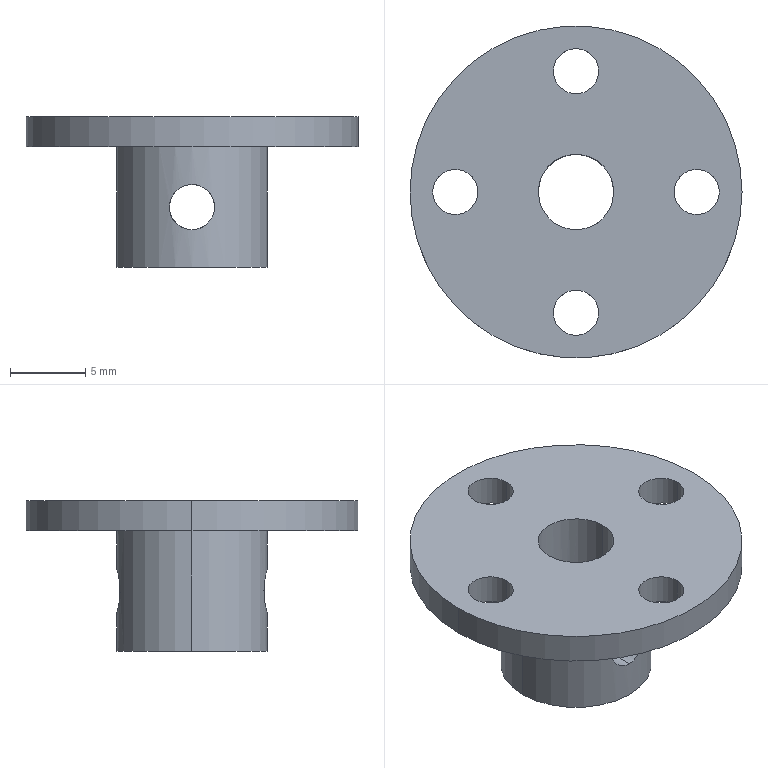Part | SolidWorks | features ICE 4, Extrusion 1 | 1 solid | 21 faces | box 22 x 22 x 10 mm | volume 1099 mm3 | cylinder 18 | plane 3 | commonest cylinder face diameters 3 x12 5 x2 10 x2 22 x2
STEP:
#1=CARTESIAN_POINT('',(0.,-5.,-5.5));
#2=VERTEX_POINT('',#1);
#3=CARTESIAN_POINT('',(0.,-5.,-2.5));
#4=VERTEX_POINT('',#3);
#5=CARTESIAN_POINT('',(0.,-5.,-5.5));
#6=CARTESIAN_POINT('',(-0.1965,-5.,-5.5));
#7=CARTESIAN_POINT('',(-0.3949,-4.988,-5.46));
#8=CARTESIAN_POINT('',(-0.6661,-4.956,-5.348));
#9=CARTESIAN_POINT('',(-0.7539,-4.944,-5.3));
#10=CARTESIAN_POINT('',(-0.9162,-4.916,-5.192));
#11=CARTESIAN_POINT('',(-0.9913,-4.901,-5.13));
#12=CARTESIAN_POINT('',(-1.199,-4.856,-4.922));
#13=CARTESIAN_POINT('',(-1.309,-4.826,-4.759));
#14=CARTESIAN_POINT('',(-1.423,-4.793,-4.485));
#15=CARTESIAN_POINT('',(-1.451,-4.785,-4.391));
#16=CARTESIAN_POINT('',(-1.49,-4.773,-4.199));
#17=CARTESIAN_POINT('',(-1.5,-4.77,-4.099));
#18=CARTESIAN_POINT('',(-1.5,-4.77,-3.901));
#19=CARTESIAN_POINT('',(-1.49,-4.773,-3.804));
#20=CARTESIAN_POINT('',(-1.452,-4.785,-3.61));
#21=CARTESIAN_POINT('',(-1.423,-4.793,-3.515));
#22=CARTESIAN_POINT('',(-1.31,-4.826,-3.244));
#23=CARTESIAN_POINT('',(-1.199,-4.856,-3.077));
#24=CARTESIAN_POINT('',(-0.9924,-4.901,-2.871));
#25=CARTESIAN_POINT('',(-0.9159,-4.916,-2.808));
#26=CARTESIAN_POINT('',(-0.7533,-4.944,-2.699));
#27=CARTESIAN_POINT('',(-0.6674,-4.956,-2.653));
#28=CARTESIAN_POINT('',(-0.4865,-4.977,-2.578));
#29=CARTESIAN_POINT('',(-0.3907,-4.986,-2.548));
#30=CARTESIAN_POINT('',(-0.1978,-4.997,-2.51));
#31=CARTESIAN_POINT('',(-0.0997,-5.,-2.5));
#32=CARTESIAN_POINT('',(0.,-5.,-2.5));
#33=B_SPLINE_CURVE_WITH_KNOTS('',3,(#5,#6,#7,#8,#9,#10,#11,#12,#13,#14,#15,#16,#17,#18,#19,#20,#21,#22,#23,#24,#25,#26,#27,#28,#29,#30,#31,#32),.UNSPECIFIED.,.F.,.F.,(4,2,2,2,2,2,2,2,2,2,2,2,2,4),(0.004717,0.005306,0.005601,0.005896,0.006485,0.00678,0.007075,0.00737,0.007664,0.008254,0.008549,0.008843,0.009138,0.009433),.UNSPECIFIED.);
#34=EDGE_CURVE('',#2,#4,#33,.T.);
#35=ORIENTED_EDGE('',*,*,#34,.F.);
#36=CARTESIAN_POINT('',(0.,-2.5,-5.5));
#37=VERTEX_POINT('',#36);
#38=CARTESIAN_POINT('',(0.,-7.,-5.5));
#39=DIRECTION('',(0.,1.,0.));
#40=VECTOR('',#39,1000.);
#41=LINE('',#38,#40);
#42=EDGE_CURVE('',#2,#37,#41,.T.);
#43=ORIENTED_EDGE('',*,*,#42,.T.);
#44=CARTESIAN_POINT('',(0.,-2.5,-2.5));
#45=VERTEX_POINT('',#44);
#46=CARTESIAN_POINT('',(0.,-2.5,-2.5));
#47=CARTESIAN_POINT('',(-0.1019,-2.5,-2.5));
#48=CARTESIAN_POINT('',(-0.2016,-2.494,-2.51));
#49=CARTESIAN_POINT('',(-0.397,-2.47,-2.55));
#50=CARTESIAN_POINT('',(-0.4936,-2.453,-2.58));
#51=CARTESIAN_POINT('',(-0.7651,-2.387,-2.695));
#52=CARTESIAN_POINT('',(-0.9278,-2.326,-2.806));
#53=CARTESIAN_POINT('',(-1.197,-2.2,-3.076));
#54=CARTESIAN_POINT('',(-1.306,-2.133,-3.238));
#55=CARTESIAN_POINT('',(-1.458,-2.033,-3.596));
#56=CARTESIAN_POINT('',(-1.5,-2.,-3.796));
#57=CARTESIAN_POINT('',(-1.5,-2.,-4.101));
#58=CARTESIAN_POINT('',(-1.49,-2.008,-4.201));
#59=CARTESIAN_POINT('',(-1.45,-2.037,-4.397));
#60=CARTESIAN_POINT('',(-1.42,-2.058,-4.492));
#61=CARTESIAN_POINT('',(-1.307,-2.133,-4.762));
#62=CARTESIAN_POINT('',(-1.197,-2.2,-4.923));
#63=CARTESIAN_POINT('',(-0.9265,-2.327,-5.195));
#64=CARTESIAN_POINT('',(-0.7662,-2.387,-5.305));
#65=CARTESIAN_POINT('',(-0.4014,-2.475,-5.459));
#66=CARTESIAN_POINT('',(-0.203,-2.5,-5.5));
#67=CARTESIAN_POINT('',(0.,-2.5,-5.5));
#68=B_SPLINE_CURVE_WITH_KNOTS('',3,(#46,#47,#48,#49,#50,#51,#52,#53,#54,#55,#56,#57,#58,#59,#60,#61,#62,#63,#64,#65,#66,#67),.UNSPECIFIED.,.F.,.F.,(4,2,2,2,2,2,2,2,2,2,4),(0.,0.0003008,0.0006015,0.001203,0.001805,0.002406,0.002707,0.003008,0.003609,0.004211,0.004812),.UNSPECIFIED.);
#69=EDGE_CURVE('',#45,#37,#68,.T.);
#70=ORIENTED_EDGE('',*,*,#69,.F.);
#71=CARTESIAN_POINT('',(0.,-7.,-2.5));
#72=DIRECTION('',(0.,1.,0.));
#73=VECTOR('',#72,1000.);
#74=LINE('',#71,#73);
#75=EDGE_CURVE('',#4,#45,#74,.T.);
#76=ORIENTED_EDGE('',*,*,#75,.F.);
#77=EDGE_LOOP('',(#35,#43,#70,#76));
#78=FACE_OUTER_BOUND('',#77,.T.);
#79=CARTESIAN_POINT('',(0.,-7.,-4.));
#80=DIRECTION('',(0.,1.,0.));
#81=DIRECTION('',(0.,0.,1.));
#82=AXIS2_PLACEMENT_3D('',#79,#80,#81);
#83=CYLINDRICAL_SURFACE('',#82,1.5);
#84=ADVANCED_FACE('',(#78),#83,.F.);
#85=CARTESIAN_POINT('',(0.,2.5,-5.5));
#86=VERTEX_POINT('',#85);
#87=CARTESIAN_POINT('',(0.,2.5,-2.5));
#88=VERTEX_POINT('',#87);
#89=CARTESIAN_POINT('',(0.,2.5,-5.5));
#90=CARTESIAN_POINT('',(-0.1013,2.5,-5.5));
#91=CARTESIAN_POINT('',(-0.2009,2.494,-5.49));
#92=CARTESIAN_POINT('',(-0.3969,2.47,-5.45));
#93=CARTESIAN_POINT('',(-0.4933,2.453,-5.42));
#94=CARTESIAN_POINT('',(-0.7647,2.387,-5.305));
#95=CARTESIAN_POINT('',(-0.9274,2.326,-5.194));
#96=CARTESIAN_POINT('',(-1.13,2.231,-4.991));
#97=CARTESIAN_POINT('',(-1.191,2.199,-4.916));
#98=CARTESIAN_POINT('',(-1.298,2.137,-4.758));
#99=CARTESIAN_POINT('',(-1.344,2.109,-4.673));
#100=CARTESIAN_POINT('',(-1.42,2.058,-4.493));
#101=CARTESIAN_POINT('',(-1.45,2.037,-4.398));
#102=CARTESIAN_POINT('',(-1.49,2.008,-4.203));
#103=CARTESIAN_POINT('',(-1.5,2.,-4.101));
#104=CARTESIAN_POINT('',(-1.5,2.,-3.799));
#105=CARTESIAN_POINT('',(-1.458,2.033,-3.598));
#106=CARTESIAN_POINT('',(-1.345,2.108,-3.328));
#107=CARTESIAN_POINT('',(-1.298,2.138,-3.242));
#108=CARTESIAN_POINT('',(-1.191,2.199,-3.083));
#109=CARTESIAN_POINT('',(-1.13,2.231,-3.009));
#110=CARTESIAN_POINT('',(-0.9258,2.327,-2.804));
#111=CARTESIAN_POINT('',(-0.7657,2.387,-2.695));
#112=CARTESIAN_POINT('',(-0.4926,2.453,-2.58));
#113=CARTESIAN_POINT('',(-0.3985,2.47,-2.55));
#114=CARTESIAN_POINT('',(-0.2037,2.494,-2.511));
#115=CARTESIAN_POINT('',(-0.1017,2.5,-2.5));
#116=CARTESIAN_POINT('',(0.,2.5,-2.5));
#117=B_SPLINE_CURVE_WITH_KNOTS('',3,(#89,#90,#91,#92,#93,#94,#95,#96,#97,#98,#99,#100,#101,#102,#103,#104,#105,#106,#107,#108,#109,#110,#111,#112,#113,#114,#115,#116),.UNSPECIFIED.,.F.,.F.,(4,2,2,2,2,2,2,2,2,2,2,2,2,4),(0.004812,0.005113,0.005413,0.006013,0.006313,0.006613,0.006914,0.007214,0.007814,0.008114,0.008415,0.009015,0.009315,0.009615),.UNSPECIFIED.);
#118=EDGE_CURVE('',#86,#88,#117,.T.);
#119=ORIENTED_EDGE('',*,*,#118,.F.);
#120=CARTESIAN_POINT('',(0.,5.,-5.5));
#121=VERTEX_POINT('',#120);
#122=CARTESIAN_POINT('',(0.,-7.,-5.5));
#123=DIRECTION('',(0.,1.,0.));
#124=VECTOR('',#123,1000.);
#125=LINE('',#122,#124);
#126=EDGE_CURVE('',#86,#121,#125,.T.);
#127=ORIENTED_EDGE('',*,*,#126,.T.);
#128=CARTESIAN_POINT('',(0.,5.,-2.5));
#129=VERTEX_POINT('',#128);
#130=CARTESIAN_POINT('',(0.,5.,-2.5));
#131=CARTESIAN_POINT('',(-0.09973,5.,-2.5));
#132=CARTESIAN_POINT('',(-0.1977,4.997,-2.51));
#133=CARTESIAN_POINT('',(-0.3902,4.986,-2.548));
#134=CARTESIAN_POINT('',(-0.4858,4.977,-2.577));
#135=CARTESIAN_POINT('',(-0.6672,4.956,-2.653));
#136=CARTESIAN_POINT('',(-0.7532,4.944,-2.699));
#137=CARTESIAN_POINT('',(-0.9158,4.916,-2.808));
#138=CARTESIAN_POINT('',(-0.9923,4.901,-2.871));
#139=CARTESIAN_POINT('',(-1.199,4.856,-3.077));
#140=CARTESIAN_POINT('',(-1.31,4.826,-3.244));
#141=CARTESIAN_POINT('',(-1.46,4.783,-3.604));
#142=CARTESIAN_POINT('',(-1.5,4.77,-3.802));
#143=CARTESIAN_POINT('',(-1.5,4.77,-4.098));
#144=CARTESIAN_POINT('',(-1.49,4.773,-4.198));
#145=CARTESIAN_POINT('',(-1.452,4.785,-4.391));
#146=CARTESIAN_POINT('',(-1.423,4.793,-4.485));
#147=CARTESIAN_POINT('',(-1.309,4.826,-4.758));
#148=CARTESIAN_POINT('',(-1.199,4.856,-4.923));
#149=CARTESIAN_POINT('',(-0.9911,4.901,-5.13));
#150=CARTESIAN_POINT('',(-0.9159,4.916,-5.192));
#151=CARTESIAN_POINT('',(-0.7538,4.944,-5.3));
#152=CARTESIAN_POINT('',(-0.666,4.956,-5.348));
#153=CARTESIAN_POINT('',(-0.4851,4.977,-5.423));
#154=CARTESIAN_POINT('',(-0.3916,4.986,-5.451));
#155=CARTESIAN_POINT('',(-0.1978,4.997,-5.49));
#156=CARTESIAN_POINT('',(-0.09827,5.,-5.5));
#157=CARTESIAN_POINT('',(0.,5.,-5.5));
#158=B_SPLINE_CURVE_WITH_KNOTS('',3,(#130,#131,#132,#133,#134,#135,#136,#137,#138,#139,#140,#141,#142,#143,#144,#145,#146,#147,#148,#149,#150,#151,#152,#153,#154,#155,#156,#157),.UNSPECIFIED.,.F.,.F.,(4,2,2,2,2,2,2,2,2,2,2,2,2,4),(0.,0.0002948,0.0005896,0.0008844,0.001179,0.001769,0.002359,0.002653,0.002948,0.003538,0.003833,0.004127,0.004422,0.004717),.UNSPECIFIED.);
#159=EDGE_CURVE('',#129,#121,#158,.T.);
#160=ORIENTED_EDGE('',*,*,#159,.F.);
#161=CARTESIAN_POINT('',(0.,-7.,-2.5));
#162=DIRECTION('',(0.,1.,0.));
#163=VECTOR('',#162,1000.);
#164=LINE('',#161,#163);
#165=EDGE_CURVE('',#88,#129,#164,.T.);
#166=ORIENTED_EDGE('',*,*,#165,.F.);
#167=EDGE_LOOP('',(#119,#127,#160,#166));
#168=FACE_OUTER_BOUND('',#167,.T.);
#169=CARTESIAN_POINT('',(0.,-7.,-4.));
#170=DIRECTION('',(0.,1.,0.));
#171=DIRECTION('',(0.,0.,1.));
#172=AXIS2_PLACEMENT_3D('',#169,#170,#171);
#173=CYLINDRICAL_SURFACE('',#172,1.5);
#174=ADVANCED_FACE('',(#168),#173,.F.);
#175=CARTESIAN_POINT('',(-1.5,-8.,0.));
#176=VERTEX_POINT('',#175);
#177=CARTESIAN_POINT('',(1.5,-8.,0.));
#178=VERTEX_POINT('',#177);
#179=CARTESIAN_POINT('',(0.,-8.,0.));
#180=DIRECTION('',(0.,0.,1.));
#181=DIRECTION('',(1.,0.,0.));
#182=AXIS2_PLACEMENT_3D('',#179,#180,#181);
#183=CIRCLE('',#182,1.5);
#184=EDGE_CURVE('',#176,#178,#183,.T.);
#185=ORIENTED_EDGE('',*,*,#184,.F.);
#186=CARTESIAN_POINT('',(-1.5,-8.,2.));
#187=VERTEX_POINT('',#186);
#188=CARTESIAN_POINT('',(-1.5,-8.,-8.));
#189=DIRECTION('',(0.,0.,1.));
#190=VECTOR('',#189,1000.);
#191=LINE('',#188,#190);
#192=EDGE_CURVE('',#176,#187,#191,.T.);
#193=ORIENTED_EDGE('',*,*,#192,.T.);
#194=CARTESIAN_POINT('',(1.5,-8.,2.));
#195=VERTEX_POINT('',#194);
#196=CARTESIAN_POINT('',(0.,-8.,2.));
#197=DIRECTION('',(0.,0.,1.));
#198=DIRECTION('',(1.,0.,0.));
#199=AXIS2_PLACEMENT_3D('',#196,#197,#198);
#200=CIRCLE('',#199,1.5);
#201=EDGE_CURVE('',#187,#195,#200,.T.);
#202=ORIENTED_EDGE('',*,*,#201,.T.);
#203=CARTESIAN_POINT('',(1.5,-8.,-8.));
#204=DIRECTION('',(0.,0.,1.));
#205=VECTOR('',#204,1000.);
#206=LINE('',#203,#205);
#207=EDGE_CURVE('',#178,#195,#206,.T.);
#208=ORIENTED_EDGE('',*,*,#207,.F.);
#209=EDGE_LOOP('',(#185,#193,#202,#208));
#210=FACE_OUTER_BOUND('',#209,.T.);
#211=CARTESIAN_POINT('',(0.,-8.,-8.));
#212=DIRECTION('',(0.,0.,1.));
#213=DIRECTION('',(1.,0.,0.));
#214=AXIS2_PLACEMENT_3D('',#211,#212,#213);
#215=CYLINDRICAL_SURFACE('',#214,1.5);
#216=ADVANCED_FACE('',(#210),#215,.F.);
#217=CARTESIAN_POINT('',(-9.5,0.,0.));
#218=VERTEX_POINT('',#217);
#219=CARTESIAN_POINT('',(-6.5,0.,0.));
#220=VERTEX_POINT('',#219);
#221=CARTESIAN_POINT('',(-8.,0.,0.));
#222=DIRECTION('',(0.,0.,1.));
#223=DIRECTION('',(1.,0.,0.));
#224=AXIS2_PLACEMENT_3D('',#221,#222,#223);
#225=CIRCLE('',#224,1.5);
#226=EDGE_CURVE('',#218,#220,#225,.T.);
#227=ORIENTED_EDGE('',*,*,#226,.F.);
#228=CARTESIAN_POINT('',(-9.5,0.,2.));
#229=VERTEX_POINT('',#228);
#230=CARTESIAN_POINT('',(-9.5,0.,-8.));
#231=DIRECTION('',(0.,0.,1.));
#232=VECTOR('',#231,1000.);
#233=LINE('',#230,#232);
#234=EDGE_CURVE('',#218,#229,#233,.T.);
#235=ORIENTED_EDGE('',*,*,#234,.T.);
#236=CARTESIAN_POINT('',(-6.5,0.,2.));
#237=VERTEX_POINT('',#236);
#238=CARTESIAN_POINT('',(-8.,0.,2.));
#239=DIRECTION('',(0.,0.,1.));
#240=DIRECTION('',(1.,0.,0.));
#241=AXIS2_PLACEMENT_3D('',#238,#239,#240);
#242=CIRCLE('',#241,1.5);
#243=EDGE_CURVE('',#229,#237,#242,.T.);
#244=ORIENTED_EDGE('',*,*,#243,.T.);
#245=CARTESIAN_POINT('',(-6.5,0.,-8.));
#246=DIRECTION('',(0.,0.,1.));
#247=VECTOR('',#246,1000.);
#248=LINE('',#245,#247);
#249=EDGE_CURVE('',#220,#237,#248,.T.);
#250=ORIENTED_EDGE('',*,*,#249,.F.);
#251=EDGE_LOOP('',(#227,#235,#244,#250));
#252=FACE_OUTER_BOUND('',#251,.T.);
#253=CARTESIAN_POINT('',(-8.,0.,-8.));
#254=DIRECTION('',(0.,0.,1.));
#255=DIRECTION('',(1.,0.,0.));
#256=AXIS2_PLACEMENT_3D('',#253,#254,#255);
#257=CYLINDRICAL_SURFACE('',#256,1.5);
#258=ADVANCED_FACE('',(#252),#257,.F.);
#259=CARTESIAN_POINT('',(-1.5,8.,0.));
#260=VERTEX_POINT('',#259);
#261=CARTESIAN_POINT('',(1.5,8.,0.));
#262=VERTEX_POINT('',#261);
#263=CARTESIAN_POINT('',(0.,8.,0.));
#264=DIRECTION('',(0.,0.,1.));
#265=DIRECTION('',(1.,0.,0.));
#266=AXIS2_PLACEMENT_3D('',#263,#264,#265);
#267=CIRCLE('',#266,1.5);
#268=EDGE_CURVE('',#260,#262,#267,.T.);
#269=ORIENTED_EDGE('',*,*,#268,.F.);
#270=CARTESIAN_POINT('',(-1.5,8.,2.));
#271=VERTEX_POINT('',#270);
#272=CARTESIAN_POINT('',(-1.5,8.,-8.));
#273=DIRECTION('',(0.,0.,1.));
#274=VECTOR('',#273,1000.);
#275=LINE('',#272,#274);
#276=EDGE_CURVE('',#260,#271,#275,.T.);
#277=ORIENTED_EDGE('',*,*,#276,.T.);
#278=CARTESIAN_POINT('',(1.5,8.,2.));
#279=VERTEX_POINT('',#278);
#280=CARTESIAN_POINT('',(0.,8.,2.));
#281=DIRECTION('',(0.,0.,1.));
#282=DIRECTION('',(1.,0.,0.));
#283=AXIS2_PLACEMENT_3D('',#280,#281,#282);
#284=CIRCLE('',#283,1.5);
#285=EDGE_CURVE('',#271,#279,#284,.T.);
#286=ORIENTED_EDGE('',*,*,#285,.T.);
#287=CARTESIAN_POINT('',(1.5,8.,-8.));
#288=DIRECTION('',(0.,0.,1.));
#289=VECTOR('',#288,1000.);
#290=LINE('',#287,#289);
#291=EDGE_CURVE('',#262,#279,#290,.T.);
#292=ORIENTED_EDGE('',*,*,#291,.F.);
#293=EDGE_LOOP('',(#269,#277,#286,#292));
#294=FACE_OUTER_BOUND('',#293,.T.);
#295=CARTESIAN_POINT('',(0.,8.,-8.));
#296=DIRECTION('',(0.,0.,1.));
#297=DIRECTION('',(1.,0.,0.));
#298=AXIS2_PLACEMENT_3D('',#295,#296,#297);
#299=CYLINDRICAL_SURFACE('',#298,1.5);
#300=ADVANCED_FACE('',(#294),#299,.F.);
#301=CARTESIAN_POINT('',(6.5,0.,0.));
#302=VERTEX_POINT('',#301);
#303=CARTESIAN_POINT('',(9.5,0.,0.));
#304=VERTEX_POINT('',#303);
#305=CARTESIAN_POINT('',(8.,0.,0.));
#306=DIRECTION('',(0.,0.,1.));
#307=DIRECTION('',(1.,0.,0.));
#308=AXIS2_PLACEMENT_3D('',#305,#306,#307);
#309=CIRCLE('',#308,1.5);
#310=EDGE_CURVE('',#302,#304,#309,.T.);
#311=ORIENTED_EDGE('',*,*,#310,.F.);
#312=CARTESIAN_POINT('',(6.5,0.,2.));
#313=VERTEX_POINT('',#312);
#314=CARTESIAN_POINT('',(6.5,0.,-8.));
#315=DIRECTION('',(0.,0.,1.));
#316=VECTOR('',#315,1000.);
#317=LINE('',#314,#316);
#318=EDGE_CURVE('',#302,#313,#317,.T.);
#319=ORIENTED_EDGE('',*,*,#318,.T.);
#320=CARTESIAN_POINT('',(9.5,0.,2.));
#321=VERTEX_POINT('',#320);
#322=CARTESIAN_POINT('',(8.,0.,2.));
#323=DIRECTION('',(0.,0.,1.));
#324=DIRECTION('',(1.,0.,0.));
#325=AXIS2_PLACEMENT_3D('',#322,#323,#324);
#326=CIRCLE('',#325,1.5);
#327=EDGE_CURVE('',#313,#321,#326,.T.);
#328=ORIENTED_EDGE('',*,*,#327,.T.);
#329=CARTESIAN_POINT('',(9.5,0.,-8.));
#330=DIRECTION('',(0.,0.,1.));
#331=VECTOR('',#330,1000.);
#332=LINE('',#329,#331);
#333=EDGE_CURVE('',#304,#321,#332,.T.);
#334=ORIENTED_EDGE('',*,*,#333,.F.);
#335=EDGE_LOOP('',(#311,#319,#328,#334));
#336=FACE_OUTER_BOUND('',#335,.T.);
#337=CARTESIAN_POINT('',(8.,0.,-8.));
#338=DIRECTION('',(0.,0.,1.));
#339=DIRECTION('',(1.,0.,0.));
#340=AXIS2_PLACEMENT_3D('',#337,#338,#339);
#341=CYLINDRICAL_SURFACE('',#340,1.5);
#342=ADVANCED_FACE('',(#336),#341,.F.);
#343=ORIENTED_EDGE('',*,*,#69,.T.);
#344=CARTESIAN_POINT('',(0.,-2.5,-5.5));
#345=CARTESIAN_POINT('',(0.1013,-2.5,-5.5));
#346=CARTESIAN_POINT('',(0.2009,-2.494,-5.49));
#347=CARTESIAN_POINT('',(0.3969,-2.47,-5.45));
#348=CARTESIAN_POINT('',(0.4933,-2.453,-5.42));
#349=CARTESIAN_POINT('',(0.7647,-2.387,-5.305));
#350=CARTESIAN_POINT('',(0.9274,-2.326,-5.194));
#351=CARTESIAN_POINT('',(1.13,-2.231,-4.991));
#352=CARTESIAN_POINT('',(1.191,-2.199,-4.916));
#353=CARTESIAN_POINT('',(1.298,-2.137,-4.758));
#354=CARTESIAN_POINT('',(1.344,-2.109,-4.673));
#355=CARTESIAN_POINT('',(1.42,-2.058,-4.493));
#356=CARTESIAN_POINT('',(1.45,-2.037,-4.398));
#357=CARTESIAN_POINT('',(1.49,-2.008,-4.203));
#358=CARTESIAN_POINT('',(1.5,-2.,-4.101));
#359=CARTESIAN_POINT('',(1.5,-2.,-3.799));
#360=CARTESIAN_POINT('',(1.458,-2.033,-3.598));
#361=CARTESIAN_POINT('',(1.345,-2.108,-3.328));
#362=CARTESIAN_POINT('',(1.298,-2.138,-3.242));
#363=CARTESIAN_POINT('',(1.191,-2.199,-3.083));
#364=CARTESIAN_POINT('',(1.13,-2.231,-3.009));
#365=CARTESIAN_POINT('',(0.9258,-2.327,-2.804));
#366=CARTESIAN_POINT('',(0.7657,-2.387,-2.695));
#367=CARTESIAN_POINT('',(0.4926,-2.453,-2.58));
#368=CARTESIAN_POINT('',(0.3985,-2.47,-2.55));
#369=CARTESIAN_POINT('',(0.2037,-2.494,-2.511));
#370=CARTESIAN_POINT('',(0.1017,-2.5,-2.5));
#371=CARTESIAN_POINT('',(0.,-2.5,-2.5));
#372=B_SPLINE_CURVE_WITH_KNOTS('',3,(#344,#345,#346,#347,#348,#349,#350,#351,#352,#353,#354,#355,#356,#357,#358,#359,#360,#361,#362,#363,#364,#365,#366,#367,#368,#369,#370,#371),.UNSPECIFIED.,.F.,.F.,(4,2,2,2,2,2,2,2,2,2,2,2,2,4),(0.004812,0.005113,0.005413,0.006013,0.006313,0.006613,0.006914,0.007214,0.007814,0.008114,0.008415,0.009015,0.009315,0.009615),.UNSPECIFIED.);
#373=EDGE_CURVE('',#37,#45,#372,.T.);
#374=ORIENTED_EDGE('',*,*,#373,.T.);
#375=EDGE_LOOP('',(#343,#374));
#376=FACE_BOUND('',#375,.T.);
#377=CARTESIAN_POINT('',(2.5,0.,2.));
#378=VERTEX_POINT('',#377);
#379=CARTESIAN_POINT('',(-2.5,0.,2.));
#380=VERTEX_POINT('',#379);
#381=CARTESIAN_POINT('',(0.,0.,2.));
#382=DIRECTION('',(0.,0.,-1.));
#383=DIRECTION('',(-1.,0.,0.));
#384=AXIS2_PLACEMENT_3D('',#381,#382,#383);
#385=CIRCLE('',#384,2.5);
#386=EDGE_CURVE('',#378,#380,#385,.T.);
#387=ORIENTED_EDGE('',*,*,#386,.F.);
#388=CARTESIAN_POINT('',(2.5,0.,-8.));
#389=VERTEX_POINT('',#388);
#390=CARTESIAN_POINT('',(2.5,0.,2.));
#391=DIRECTION('',(0.,0.,-1.));
#392=VECTOR('',#391,1000.);
#393=LINE('',#390,#392);
#394=EDGE_CURVE('',#378,#389,#393,.T.);
#395=ORIENTED_EDGE('',*,*,#394,.T.);
#396=CARTESIAN_POINT('',(-2.5,0.,-8.));
#397=VERTEX_POINT('',#396);
#398=CARTESIAN_POINT('',(0.,0.,-8.));
#399=DIRECTION('',(0.,0.,-1.));
#400=DIRECTION('',(-1.,0.,0.));
#401=AXIS2_PLACEMENT_3D('',#398,#399,#400);
#402=CIRCLE('',#401,2.5);
#403=EDGE_CURVE('',#389,#397,#402,.T.);
#404=ORIENTED_EDGE('',*,*,#403,.T.);
#405=CARTESIAN_POINT('',(-2.5,0.,2.));
#406=DIRECTION('',(0.,0.,-1.));
#407=VECTOR('',#406,1000.);
#408=LINE('',#405,#407);
#409=EDGE_CURVE('',#380,#397,#408,.T.);
#410=ORIENTED_EDGE('',*,*,#409,.F.);
#411=EDGE_LOOP('',(#387,#395,#404,#410));
#412=FACE_OUTER_BOUND('',#411,.T.);
#413=CARTESIAN_POINT('',(0.,0.,2.));
#414=DIRECTION('',(0.,0.,-1.));
#415=DIRECTION('',(-1.,0.,0.));
#416=AXIS2_PLACEMENT_3D('',#413,#414,#415);
#417=CYLINDRICAL_SURFACE('',#416,2.5);
#418=ADVANCED_FACE('',(#376,#412),#417,.F.);
#419=ORIENTED_EDGE('',*,*,#159,.T.);
#420=CARTESIAN_POINT('',(0.,5.,-5.5));
#421=CARTESIAN_POINT('',(0.1965,5.,-5.5));
#422=CARTESIAN_POINT('',(0.3949,4.988,-5.46));
#423=CARTESIAN_POINT('',(0.6661,4.956,-5.348));
#424=CARTESIAN_POINT('',(0.7539,4.944,-5.3));
#425=CARTESIAN_POINT('',(0.9162,4.916,-5.192));
#426=CARTESIAN_POINT('',(0.9913,4.901,-5.13));
#427=CARTESIAN_POINT('',(1.199,4.856,-4.922));
#428=CARTESIAN_POINT('',(1.309,4.826,-4.759));
#429=CARTESIAN_POINT('',(1.423,4.793,-4.485));
#430=CARTESIAN_POINT('',(1.451,4.785,-4.391));
#431=CARTESIAN_POINT('',(1.49,4.773,-4.199));
#432=CARTESIAN_POINT('',(1.5,4.77,-4.099));
#433=CARTESIAN_POINT('',(1.5,4.77,-3.901));
#434=CARTESIAN_POINT('',(1.49,4.773,-3.804));
#435=CARTESIAN_POINT('',(1.452,4.785,-3.61));
#436=CARTESIAN_POINT('',(1.423,4.793,-3.515));
#437=CARTESIAN_POINT('',(1.31,4.826,-3.244));
#438=CARTESIAN_POINT('',(1.199,4.856,-3.077));
#439=CARTESIAN_POINT('',(0.9924,4.901,-2.871));
#440=CARTESIAN_POINT('',(0.9159,4.916,-2.808));
#441=CARTESIAN_POINT('',(0.7533,4.944,-2.699));
#442=CARTESIAN_POINT('',(0.6674,4.956,-2.653));
#443=CARTESIAN_POINT('',(0.4865,4.977,-2.578));
#444=CARTESIAN_POINT('',(0.3907,4.986,-2.548));
#445=CARTESIAN_POINT('',(0.1978,4.997,-2.51));
#446=CARTESIAN_POINT('',(0.0997,5.,-2.5));
#447=CARTESIAN_POINT('',(0.,5.,-2.5));
#448=B_SPLINE_CURVE_WITH_KNOTS('',3,(#420,#421,#422,#423,#424,#425,#426,#427,#428,#429,#430,#431,#432,#433,#434,#435,#436,#437,#438,#439,#440,#441,#442,#443,#444,#445,#446,#447),.UNSPECIFIED.,.F.,.F.,(4,2,2,2,2,2,2,2,2,2,2,2,2,4),(0.004717,0.005306,0.005601,0.005896,0.006485,0.00678,0.007075,0.00737,0.007664,0.008254,0.008549,0.008843,0.009138,0.009433),.UNSPECIFIED.);
#449=EDGE_CURVE('',#121,#129,#448,.T.);
#450=ORIENTED_EDGE('',*,*,#449,.T.);
#451=EDGE_LOOP('',(#419,#450));
#452=FACE_BOUND('',#451,.T.);
#453=CARTESIAN_POINT('',(-5.,0.,-8.));
#454=VERTEX_POINT('',#453);
#455=CARTESIAN_POINT('',(5.,0.,-8.));
#456=VERTEX_POINT('',#455);
#457=CARTESIAN_POINT('',(0.,0.,-8.));
#458=DIRECTION('',(0.,0.,-1.));
#459=DIRECTION('',(-1.,0.,0.));
#460=AXIS2_PLACEMENT_3D('',#457,#458,#459);
#461=CIRCLE('',#460,5.);
#462=EDGE_CURVE('',#454,#456,#461,.T.);
#463=ORIENTED_EDGE('',*,*,#462,.F.);
#464=CARTESIAN_POINT('',(-5.,0.,0.));
#465=VERTEX_POINT('',#464);
#466=CARTESIAN_POINT('',(-5.,0.,-8.));
#467=DIRECTION('',(0.,0.,1.));
#468=VECTOR('',#467,1000.);
#469=LINE('',#466,#468);
#470=EDGE_CURVE('',#454,#465,#469,.T.);
#471=ORIENTED_EDGE('',*,*,#470,.T.);
#472=CARTESIAN_POINT('',(5.,0.,0.));
#473=VERTEX_POINT('',#472);
#474=CARTESIAN_POINT('',(0.,0.,0.));
#475=DIRECTION('',(0.,0.,-1.));
#476=DIRECTION('',(-1.,0.,0.));
#477=AXIS2_PLACEMENT_3D('',#474,#475,#476);
#478=CIRCLE('',#477,5.);
#479=EDGE_CURVE('',#465,#473,#478,.T.);
#480=ORIENTED_EDGE('',*,*,#479,.T.);
#481=CARTESIAN_POINT('',(5.,0.,-8.));
#482=DIRECTION('',(0.,0.,1.));
#483=VECTOR('',#482,1000.);
#484=LINE('',#481,#483);
#485=EDGE_CURVE('',#456,#473,#484,.T.);
#486=ORIENTED_EDGE('',*,*,#485,.F.);
#487=EDGE_LOOP('',(#463,#471,#480,#486));
#488=FACE_OUTER_BOUND('',#487,.T.);
#489=CARTESIAN_POINT('',(0.,0.,-8.));
#490=DIRECTION('',(0.,0.,1.));
#491=DIRECTION('',(1.,0.,0.));
#492=AXIS2_PLACEMENT_3D('',#489,#490,#491);
#493=CYLINDRICAL_SURFACE('',#492,5.);
#494=ADVANCED_FACE('',(#452,#488),#493,.T.);
#495=CARTESIAN_POINT('',(11.,0.,2.));
#496=VERTEX_POINT('',#495);
#497=CARTESIAN_POINT('',(-11.,0.,2.));
#498=VERTEX_POINT('',#497);
#499=CARTESIAN_POINT('',(0.,0.,2.));
#500=DIRECTION('',(0.,0.,1.));
#501=DIRECTION('',(1.,0.,0.));
#502=AXIS2_PLACEMENT_3D('',#499,#500,#501);
#503=CIRCLE('',#502,11.);
#504=EDGE_CURVE('',#496,#498,#503,.T.);
#505=ORIENTED_EDGE('',*,*,#504,.F.);
#506=CARTESIAN_POINT('',(11.,0.,0.));
#507=VERTEX_POINT('',#506);
#508=CARTESIAN_POINT('',(11.,0.,2.));
#509=DIRECTION('',(0.,0.,-1.));
#510=VECTOR('',#509,1000.);
#511=LINE('',#508,#510);
#512=EDGE_CURVE('',#496,#507,#511,.T.);
#513=ORIENTED_EDGE('',*,*,#512,.T.);
#514=CARTESIAN_POINT('',(-11.,0.,0.));
#515=VERTEX_POINT('',#514);
#516=CARTESIAN_POINT('',(0.,0.,0.));
#517=DIRECTION('',(0.,0.,1.));
#518=DIRECTION('',(1.,0.,0.));
#519=AXIS2_PLACEMENT_3D('',#516,#517,#518);
#520=CIRCLE('',#519,11.);
#521=EDGE_CURVE('',#507,#515,#520,.T.);
#522=ORIENTED_EDGE('',*,*,#521,.T.);
#523=CARTESIAN_POINT('',(-11.,0.,2.));
#524=DIRECTION('',(0.,0.,-1.));
#525=VECTOR('',#524,1000.);
#526=LINE('',#523,#525);
#527=EDGE_CURVE('',#498,#515,#526,.T.);
#528=ORIENTED_EDGE('',*,*,#527,.F.);
#529=EDGE_LOOP('',(#505,#513,#522,#528));
#530=FACE_OUTER_BOUND('',#529,.T.);
#531=CARTESIAN_POINT('',(0.,0.,2.));
#532=DIRECTION('',(0.,0.,-1.));
#533=DIRECTION('',(-1.,0.,0.));
#534=AXIS2_PLACEMENT_3D('',#531,#532,#533);
#535=CYLINDRICAL_SURFACE('',#534,11.);
#536=ADVANCED_FACE('',(#530),#535,.T.);
#537=ORIENTED_EDGE('',*,*,#512,.F.);
#538=CARTESIAN_POINT('',(0.,0.,2.));
#539=DIRECTION('',(0.,0.,1.));
#540=DIRECTION('',(1.,0.,0.));
#541=AXIS2_PLACEMENT_3D('',#538,#539,#540);
#542=CIRCLE('',#541,11.);
#543=EDGE_CURVE('',#498,#496,#542,.T.);
#544=ORIENTED_EDGE('',*,*,#543,.F.);
#545=ORIENTED_EDGE('',*,*,#527,.T.);
#546=CARTESIAN_POINT('',(0.,0.,0.));
#547=DIRECTION('',(0.,0.,1.));
#548=DIRECTION('',(1.,0.,0.));
#549=AXIS2_PLACEMENT_3D('',#546,#547,#548);
#550=CIRCLE('',#549,11.);
#551=EDGE_CURVE('',#515,#507,#550,.T.);
#552=ORIENTED_EDGE('',*,*,#551,.T.);
#553=EDGE_LOOP('',(#537,#544,#545,#552));
#554=FACE_OUTER_BOUND('',#553,.T.);
#555=CARTESIAN_POINT('',(0.,0.,2.));
#556=DIRECTION('',(0.,0.,-1.));
#557=DIRECTION('',(-1.,0.,0.));
#558=AXIS2_PLACEMENT_3D('',#555,#556,#557);
#559=CYLINDRICAL_SURFACE('',#558,11.);
#560=ADVANCED_FACE('',(#554),#559,.T.);
#561=CARTESIAN_POINT('',(0.,-8.,2.));
#562=DIRECTION('',(0.,0.,1.));
#563=DIRECTION('',(1.,0.,0.));
#564=AXIS2_PLACEMENT_3D('',#561,#562,#563);
#565=CIRCLE('',#564,1.5);
#566=EDGE_CURVE('',#195,#187,#565,.T.);
#567=ORIENTED_EDGE('',*,*,#566,.F.);
#568=ORIENTED_EDGE('',*,*,#201,.F.);
#569=EDGE_LOOP('',(#567,#568));
#570=FACE_BOUND('',#569,.T.);
#571=CARTESIAN_POINT('',(-8.,0.,2.));
#572=DIRECTION('',(0.,0.,1.));
#573=DIRECTION('',(1.,0.,0.));
#574=AXIS2_PLACEMENT_3D('',#571,#572,#573);
#575=CIRCLE('',#574,1.5);
#576=EDGE_CURVE('',#237,#229,#575,.T.);
#577=ORIENTED_EDGE('',*,*,#576,.F.);
#578=ORIENTED_EDGE('',*,*,#243,.F.);
#579=EDGE_LOOP('',(#577,#578));
#580=FACE_BOUND('',#579,.T.);
#581=CARTESIAN_POINT('',(0.,8.,2.));
#582=DIRECTION('',(0.,0.,1.));
#583=DIRECTION('',(1.,0.,0.));
#584=AXIS2_PLACEMENT_3D('',#581,#582,#583);
#585=CIRCLE('',#584,1.5);
#586=EDGE_CURVE('',#279,#271,#585,.T.);
#587=ORIENTED_EDGE('',*,*,#586,.F.);
#588=ORIENTED_EDGE('',*,*,#285,.F.);
#589=EDGE_LOOP('',(#587,#588));
#590=FACE_BOUND('',#589,.T.);
#591=CARTESIAN_POINT('',(8.,0.,2.));
#592=DIRECTION('',(0.,0.,1.));
#593=DIRECTION('',(1.,0.,0.));
#594=AXIS2_PLACEMENT_3D('',#591,#592,#593);
#595=CIRCLE('',#594,1.5);
#596=EDGE_CURVE('',#321,#313,#595,.T.);
#597=ORIENTED_EDGE('',*,*,#596,.F.);
#598=ORIENTED_EDGE('',*,*,#327,.F.);
#599=EDGE_LOOP('',(#597,#598));
#600=FACE_BOUND('',#599,.T.);
#601=CARTESIAN_POINT('',(0.,0.,2.));
#602=DIRECTION('',(0.,0.,-1.));
#603=DIRECTION('',(-1.,0.,0.));
#604=AXIS2_PLACEMENT_3D('',#601,#602,#603);
#605=CIRCLE('',#604,2.5);
#606=EDGE_CURVE('',#380,#378,#605,.T.);
#607=ORIENTED_EDGE('',*,*,#606,.T.);
#608=ORIENTED_EDGE('',*,*,#386,.T.);
#609=EDGE_LOOP('',(#607,#608));
#610=FACE_BOUND('',#609,.T.);
#611=ORIENTED_EDGE('',*,*,#543,.T.);
#612=ORIENTED_EDGE('',*,*,#504,.T.);
#613=EDGE_LOOP('',(#611,#612));
#614=FACE_OUTER_BOUND('',#613,.T.);
#615=CARTESIAN_POINT('',(0.,0.,2.));
#616=DIRECTION('',(0.,0.,1.));
#617=DIRECTION('',(1.,0.,0.));
#618=AXIS2_PLACEMENT_3D('',#615,#616,#617);
#619=PLANE('',#618);
#620=ADVANCED_FACE('',(#570,#580,#590,#600,#610,#614),#619,.T.);
#621=CARTESIAN_POINT('',(0.,-8.,0.));
#622=DIRECTION('',(0.,0.,1.));
#623=DIRECTION('',(1.,0.,0.));
#624=AXIS2_PLACEMENT_3D('',#621,#622,#623);
#625=CIRCLE('',#624,1.5);
#626=EDGE_CURVE('',#178,#176,#625,.T.);
#627=ORIENTED_EDGE('',*,*,#626,.T.);
#628=ORIENTED_EDGE('',*,*,#184,.T.);
#629=EDGE_LOOP('',(#627,#628));
#630=FACE_BOUND('',#629,.T.);
#631=CARTESIAN_POINT('',(-8.,0.,0.));
#632=DIRECTION('',(0.,0.,1.));
#633=DIRECTION('',(1.,0.,0.));
#634=AXIS2_PLACEMENT_3D('',#631,#632,#633);
#635=CIRCLE('',#634,1.5);
#636=EDGE_CURVE('',#220,#218,#635,.T.);
#637=ORIENTED_EDGE('',*,*,#636,.T.);
#638=ORIENTED_EDGE('',*,*,#226,.T.);
#639=EDGE_LOOP('',(#637,#638));
#640=FACE_BOUND('',#639,.T.);
#641=CARTESIAN_POINT('',(0.,8.,0.));
#642=DIRECTION('',(0.,0.,1.));
#643=DIRECTION('',(1.,0.,0.));
#644=AXIS2_PLACEMENT_3D('',#641,#642,#643);
#645=CIRCLE('',#644,1.5);
#646=EDGE_CURVE('',#262,#260,#645,.T.);
#647=ORIENTED_EDGE('',*,*,#646,.T.);
#648=ORIENTED_EDGE('',*,*,#268,.T.);
#649=EDGE_LOOP('',(#647,#648));
#650=FACE_BOUND('',#649,.T.);
#651=CARTESIAN_POINT('',(8.,0.,0.));
#652=DIRECTION('',(0.,0.,1.));
#653=DIRECTION('',(1.,0.,0.));
#654=AXIS2_PLACEMENT_3D('',#651,#652,#653);
#655=CIRCLE('',#654,1.5);
#656=EDGE_CURVE('',#304,#302,#655,.T.);
#657=ORIENTED_EDGE('',*,*,#656,.T.);
#658=ORIENTED_EDGE('',*,*,#310,.T.);
#659=EDGE_LOOP('',(#657,#658));
#660=FACE_BOUND('',#659,.T.);
#661=CARTESIAN_POINT('',(0.,0.,0.));
#662=DIRECTION('',(0.,0.,-1.));
#663=DIRECTION('',(-1.,0.,0.));
#664=AXIS2_PLACEMENT_3D('',#661,#662,#663);
#665=CIRCLE('',#664,5.);
#666=EDGE_CURVE('',#473,#465,#665,.T.);
#667=ORIENTED_EDGE('',*,*,#666,.F.);
#668=ORIENTED_EDGE('',*,*,#479,.F.);
#669=EDGE_LOOP('',(#667,#668));
#670=FACE_BOUND('',#669,.T.);
#671=ORIENTED_EDGE('',*,*,#551,.F.);
#672=ORIENTED_EDGE('',*,*,#521,.F.);
#673=EDGE_LOOP('',(#671,#672));
#674=FACE_OUTER_BOUND('',#673,.T.);
#675=CARTESIAN_POINT('',(0.,0.,0.));
#676=DIRECTION('',(0.,0.,1.));
#677=DIRECTION('',(1.,0.,0.));
#678=AXIS2_PLACEMENT_3D('',#675,#676,#677);
#679=PLANE('',#678);
#680=ADVANCED_FACE('',(#630,#640,#650,#660,#670,#674),#679,.F.);
#681=ORIENTED_EDGE('',*,*,#470,.F.);
#682=CARTESIAN_POINT('',(0.,0.,-8.));
#683=DIRECTION('',(0.,0.,-1.));
#684=DIRECTION('',(-1.,0.,0.));
#685=AXIS2_PLACEMENT_3D('',#682,#683,#684);
#686=CIRCLE('',#685,5.);
#687=EDGE_CURVE('',#456,#454,#686,.T.);
#688=ORIENTED_EDGE('',*,*,#687,.F.);
#689=ORIENTED_EDGE('',*,*,#485,.T.);
#690=ORIENTED_EDGE('',*,*,#666,.T.);
#691=EDGE_LOOP('',(#681,#688,#689,#690));
#692=FACE_OUTER_BOUND('',#691,.T.);
#693=CARTESIAN_POINT('',(0.,-5.,-2.5));
#694=CARTESIAN_POINT('',(0.09973,-5.,-2.5));
#695=CARTESIAN_POINT('',(0.1977,-4.997,-2.51));
#696=CARTESIAN_POINT('',(0.3902,-4.986,-2.548));
#697=CARTESIAN_POINT('',(0.4858,-4.977,-2.577));
#698=CARTESIAN_POINT('',(0.6672,-4.956,-2.653));
#699=CARTESIAN_POINT('',(0.7532,-4.944,-2.699));
#700=CARTESIAN_POINT('',(0.9158,-4.916,-2.808));
#701=CARTESIAN_POINT('',(0.9923,-4.901,-2.871));
#702=CARTESIAN_POINT('',(1.199,-4.856,-3.077));
#703=CARTESIAN_POINT('',(1.31,-4.826,-3.244));
#704=CARTESIAN_POINT('',(1.46,-4.783,-3.604));
#705=CARTESIAN_POINT('',(1.5,-4.77,-3.802));
#706=CARTESIAN_POINT('',(1.5,-4.77,-4.098));
#707=CARTESIAN_POINT('',(1.49,-4.773,-4.198));
#708=CARTESIAN_POINT('',(1.452,-4.785,-4.391));
#709=CARTESIAN_POINT('',(1.423,-4.793,-4.485));
#710=CARTESIAN_POINT('',(1.309,-4.826,-4.758));
#711=CARTESIAN_POINT('',(1.199,-4.856,-4.923));
#712=CARTESIAN_POINT('',(0.9911,-4.901,-5.13));
#713=CARTESIAN_POINT('',(0.9159,-4.916,-5.192));
#714=CARTESIAN_POINT('',(0.7538,-4.944,-5.3));
#715=CARTESIAN_POINT('',(0.666,-4.956,-5.348));
#716=CARTESIAN_POINT('',(0.4851,-4.977,-5.423));
#717=CARTESIAN_POINT('',(0.3916,-4.986,-5.451));
#718=CARTESIAN_POINT('',(0.1978,-4.997,-5.49));
#719=CARTESIAN_POINT('',(0.09827,-5.,-5.5));
#720=CARTESIAN_POINT('',(0.,-5.,-5.5));
#721=B_SPLINE_CURVE_WITH_KNOTS('',3,(#693,#694,#695,#696,#697,#698,#699,#700,#701,#702,#703,#704,#705,#706,#707,#708,#709,#710,#711,#712,#713,#714,#715,#716,#717,#718,#719,#720),.UNSPECIFIED.,.F.,.F.,(4,2,2,2,2,2,2,2,2,2,2,2,2,4),(0.,0.0002948,0.0005896,0.0008844,0.001179,0.001769,0.002359,0.002653,0.002948,0.003538,0.003833,0.004127,0.004422,0.004717),.UNSPECIFIED.);
#722=EDGE_CURVE('',#4,#2,#721,.T.);
#723=ORIENTED_EDGE('',*,*,#722,.T.);
#724=ORIENTED_EDGE('',*,*,#34,.T.);
#725=EDGE_LOOP('',(#723,#724));
#726=FACE_BOUND('',#725,.T.);
#727=CARTESIAN_POINT('',(0.,0.,-8.));
#728=DIRECTION('',(0.,0.,1.));
#729=DIRECTION('',(1.,0.,0.));
#730=AXIS2_PLACEMENT_3D('',#727,#728,#729);
#731=CYLINDRICAL_SURFACE('',#730,5.);
#732=ADVANCED_FACE('',(#692,#726),#731,.T.);
#733=CARTESIAN_POINT('',(0.,0.,-8.));
#734=DIRECTION('',(0.,0.,-1.));
#735=DIRECTION('',(-1.,0.,0.));
#736=AXIS2_PLACEMENT_3D('',#733,#734,#735);
#737=CIRCLE('',#736,2.5);
#738=EDGE_CURVE('',#397,#389,#737,.T.);
#739=ORIENTED_EDGE('',*,*,#738,.F.);
#740=ORIENTED_EDGE('',*,*,#403,.F.);
#741=EDGE_LOOP('',(#739,#740));
#742=FACE_BOUND('',#741,.T.);
#743=ORIENTED_EDGE('',*,*,#687,.T.);
#744=ORIENTED_EDGE('',*,*,#462,.T.);
#745=EDGE_LOOP('',(#743,#744));
#746=FACE_OUTER_BOUND('',#745,.T.);
#747=CARTESIAN_POINT('',(0.,0.,-8.));
#748=DIRECTION('',(0.,0.,-1.));
#749=DIRECTION('',(-1.,0.,0.));
#750=AXIS2_PLACEMENT_3D('',#747,#748,#749);
#751=PLANE('',#750);
#752=ADVANCED_FACE('',(#742,#746),#751,.T.);
#753=ORIENTED_EDGE('',*,*,#394,.F.);
#754=ORIENTED_EDGE('',*,*,#606,.F.);
#755=ORIENTED_EDGE('',*,*,#409,.T.);
#756=ORIENTED_EDGE('',*,*,#738,.T.);
#757=EDGE_LOOP('',(#753,#754,#755,#756));
#758=FACE_OUTER_BOUND('',#757,.T.);
#759=CARTESIAN_POINT('',(0.,2.5,-2.5));
#760=CARTESIAN_POINT('',(0.1019,2.5,-2.5));
#761=CARTESIAN_POINT('',(0.2016,2.494,-2.51));
#762=CARTESIAN_POINT('',(0.397,2.47,-2.55));
#763=CARTESIAN_POINT('',(0.4936,2.453,-2.58));
#764=CARTESIAN_POINT('',(0.7651,2.387,-2.695));
#765=CARTESIAN_POINT('',(0.9278,2.326,-2.806));
#766=CARTESIAN_POINT('',(1.197,2.2,-3.076));
#767=CARTESIAN_POINT('',(1.306,2.133,-3.238));
#768=CARTESIAN_POINT('',(1.458,2.033,-3.596));
#769=CARTESIAN_POINT('',(1.5,2.,-3.796));
#770=CARTESIAN_POINT('',(1.5,2.,-4.101));
#771=CARTESIAN_POINT('',(1.49,2.008,-4.201));
#772=CARTESIAN_POINT('',(1.45,2.037,-4.397));
#773=CARTESIAN_POINT('',(1.42,2.058,-4.492));
#774=CARTESIAN_POINT('',(1.307,2.133,-4.762));
#775=CARTESIAN_POINT('',(1.197,2.2,-4.923));
#776=CARTESIAN_POINT('',(0.9265,2.327,-5.195));
#777=CARTESIAN_POINT('',(0.7662,2.387,-5.305));
#778=CARTESIAN_POINT('',(0.4014,2.475,-5.459));
#779=CARTESIAN_POINT('',(0.203,2.5,-5.5));
#780=CARTESIAN_POINT('',(0.,2.5,-5.5));
#781=B_SPLINE_CURVE_WITH_KNOTS('',3,(#759,#760,#761,#762,#763,#764,#765,#766,#767,#768,#769,#770,#771,#772,#773,#774,#775,#776,#777,#778,#779,#780),.UNSPECIFIED.,.F.,.F.,(4,2,2,2,2,2,2,2,2,2,4),(0.,0.0003008,0.0006015,0.001203,0.001805,0.002406,0.002707,0.003008,0.003609,0.004211,0.004812),.UNSPECIFIED.);
#782=EDGE_CURVE('',#88,#86,#781,.T.);
#783=ORIENTED_EDGE('',*,*,#782,.T.);
#784=ORIENTED_EDGE('',*,*,#118,.T.);
#785=EDGE_LOOP('',(#783,#784));
#786=FACE_BOUND('',#785,.T.);
#787=CARTESIAN_POINT('',(0.,0.,2.));
#788=DIRECTION('',(0.,0.,-1.));
#789=DIRECTION('',(-1.,0.,0.));
#790=AXIS2_PLACEMENT_3D('',#787,#788,#789);
#791=CYLINDRICAL_SURFACE('',#790,2.5);
#792=ADVANCED_FACE('',(#758,#786),#791,.F.);
#793=ORIENTED_EDGE('',*,*,#318,.F.);
#794=ORIENTED_EDGE('',*,*,#656,.F.);
#795=ORIENTED_EDGE('',*,*,#333,.T.);
#796=ORIENTED_EDGE('',*,*,#596,.T.);
#797=EDGE_LOOP('',(#793,#794,#795,#796));
#798=FACE_OUTER_BOUND('',#797,.T.);
#799=CARTESIAN_POINT('',(8.,0.,-8.));
#800=DIRECTION('',(0.,0.,1.));
#801=DIRECTION('',(1.,0.,0.));
#802=AXIS2_PLACEMENT_3D('',#799,#800,#801);
#803=CYLINDRICAL_SURFACE('',#802,1.5);
#804=ADVANCED_FACE('',(#798),#803,.F.);
#805=ORIENTED_EDGE('',*,*,#276,.F.);
#806=ORIENTED_EDGE('',*,*,#646,.F.);
#807=ORIENTED_EDGE('',*,*,#291,.T.);
#808=ORIENTED_EDGE('',*,*,#586,.T.);
#809=EDGE_LOOP('',(#805,#806,#807,#808));
#810=FACE_OUTER_BOUND('',#809,.T.);
#811=CARTESIAN_POINT('',(0.,8.,-8.));
#812=DIRECTION('',(0.,0.,1.));
#813=DIRECTION('',(1.,0.,0.));
#814=AXIS2_PLACEMENT_3D('',#811,#812,#813);
#815=CYLINDRICAL_SURFACE('',#814,1.5);
#816=ADVANCED_FACE('',(#810),#815,.F.);
#817=ORIENTED_EDGE('',*,*,#234,.F.);
#818=ORIENTED_EDGE('',*,*,#636,.F.);
#819=ORIENTED_EDGE('',*,*,#249,.T.);
#820=ORIENTED_EDGE('',*,*,#576,.T.);
#821=EDGE_LOOP('',(#817,#818,#819,#820));
#822=FACE_OUTER_BOUND('',#821,.T.);
#823=CARTESIAN_POINT('',(-8.,0.,-8.));
#824=DIRECTION('',(0.,0.,1.));
#825=DIRECTION('',(1.,0.,0.));
#826=AXIS2_PLACEMENT_3D('',#823,#824,#825);
#827=CYLINDRICAL_SURFACE('',#826,1.5);
#828=ADVANCED_FACE('',(#822),#827,.F.);
#829=ORIENTED_EDGE('',*,*,#192,.F.);
#830=ORIENTED_EDGE('',*,*,#626,.F.);
#831=ORIENTED_EDGE('',*,*,#207,.T.);
#832=ORIENTED_EDGE('',*,*,#566,.T.);
#833=EDGE_LOOP('',(#829,#830,#831,#832));
#834=FACE_OUTER_BOUND('',#833,.T.);
#835=CARTESIAN_POINT('',(0.,-8.,-8.));
#836=DIRECTION('',(0.,0.,1.));
#837=DIRECTION('',(1.,0.,0.));
#838=AXIS2_PLACEMENT_3D('',#835,#836,#837);
#839=CYLINDRICAL_SURFACE('',#838,1.5);
#840=ADVANCED_FACE('',(#834),#839,.F.);
#841=ORIENTED_EDGE('',*,*,#126,.F.);
#842=ORIENTED_EDGE('',*,*,#782,.F.);
#843=ORIENTED_EDGE('',*,*,#165,.T.);
#844=ORIENTED_EDGE('',*,*,#449,.F.);
#845=EDGE_LOOP('',(#841,#842,#843,#844));
#846=FACE_OUTER_BOUND('',#845,.T.);
#847=CARTESIAN_POINT('',(0.,-7.,-4.));
#848=DIRECTION('',(0.,1.,0.));
#849=DIRECTION('',(0.,0.,1.));
#850=AXIS2_PLACEMENT_3D('',#847,#848,#849);
#851=CYLINDRICAL_SURFACE('',#850,1.5);
#852=ADVANCED_FACE('',(#846),#851,.F.);
#853=ORIENTED_EDGE('',*,*,#42,.F.);
#854=ORIENTED_EDGE('',*,*,#722,.F.);
#855=ORIENTED_EDGE('',*,*,#75,.T.);
#856=ORIENTED_EDGE('',*,*,#373,.F.);
#857=EDGE_LOOP('',(#853,#854,#855,#856));
#858=FACE_OUTER_BOUND('',#857,.T.);
#859=CARTESIAN_POINT('',(0.,-7.,-4.));
#860=DIRECTION('',(0.,1.,0.));
#861=DIRECTION('',(0.,0.,1.));
#862=AXIS2_PLACEMENT_3D('',#859,#860,#861);
#863=CYLINDRICAL_SURFACE('',#862,1.5);
#864=ADVANCED_FACE('',(#858),#863,.F.);
#865=CLOSED_SHELL('',(#84,#174,#216,#258,#300,#342,#418,#494,#536,#560,#620,#680,#732,#752,#792,#804,#816,#828,#840,#852,#864));
#866=MANIFOLD_SOLID_BREP('',#865);
#867=CARTESIAN_POINT('',(0.,0.,0.));
#868=DIRECTION('',(0.,0.,1.));
#869=DIRECTION('',(1.,0.,0.));
#870=AXIS2_PLACEMENT_3D('',#867,#868,#869);
#871=(LENGTH_UNIT()NAMED_UNIT(*)SI_UNIT(.MILLI.,.METRE.));
#872=UNCERTAINTY_MEASURE_WITH_UNIT(LENGTH_MEASURE(0.00001),#871,'','');
#873=(NAMED_UNIT(*)PLANE_ANGLE_UNIT()SI_UNIT($,.RADIAN.));
#874=(NAMED_UNIT(*)SI_UNIT($,.STERADIAN.)SOLID_ANGLE_UNIT());
#875=(GEOMETRIC_REPRESENTATION_CONTEXT(3)GLOBAL_UNCERTAINTY_ASSIGNED_CONTEXT((#872))GLOBAL_UNIT_ASSIGNED_CONTEXT((#871,#873,#874))REPRESENTATION_CONTEXT('',''));
#876=ADVANCED_BREP_SHAPE_REPRESENTATION('',(#866,#870),#875);